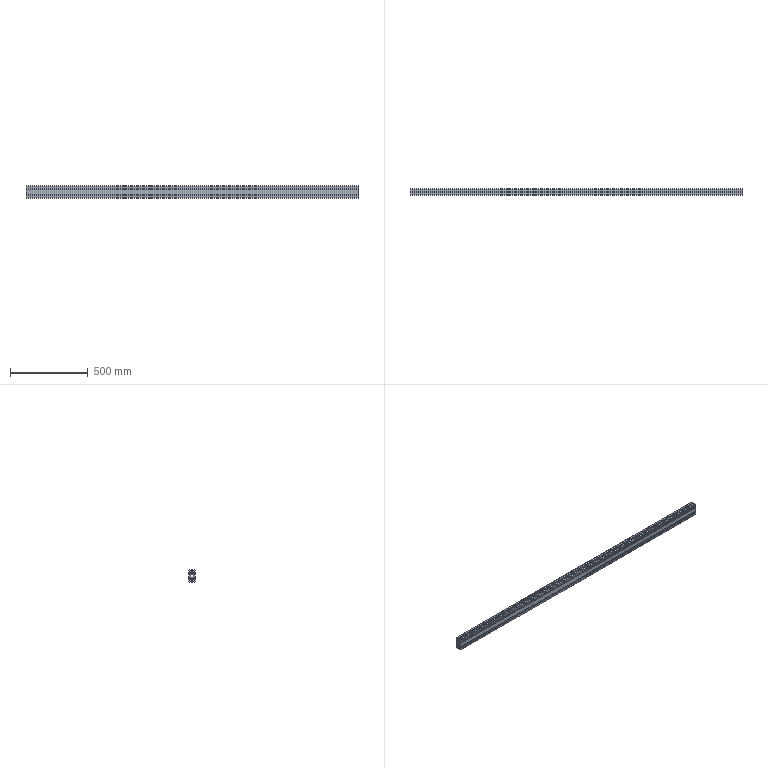Part | NX | 1 solid | 82 faces | box 2140 x 40 x 80 mm | volume 4638453 mm3 | plane 74 | cylinder 8 | commonest cylinder face diameters 6.78 x4 6.8 x4